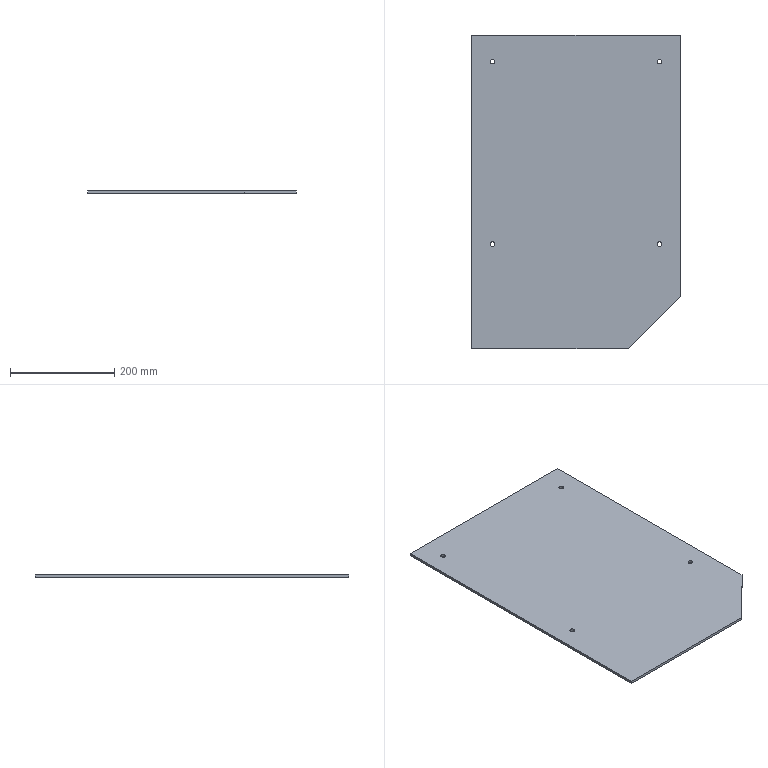Part | SolidWorks | features Chamfer 1, Extrusion 1, ICE 1 | 1 solid | 15 faces | box 400 x 600 x 5 mm | volume 1173728 mm3 | cylinder 8 | plane 7 | commonest cylinder face diameters 9 x8
STEP:
#1=CARTESIAN_POINT('',(-164.5,-100.,0.));
#2=VERTEX_POINT('',#1);
#3=CARTESIAN_POINT('',(-155.5,-100.,0.));
#4=VERTEX_POINT('',#3);
#5=CARTESIAN_POINT('',(-160.,-100.,0.));
#6=DIRECTION('',(0.,0.,1.));
#7=DIRECTION('',(1.,0.,0.));
#8=AXIS2_PLACEMENT_3D('',#5,#6,#7);
#9=CIRCLE('',#8,4.5);
#10=EDGE_CURVE('',#2,#4,#9,.T.);
#11=ORIENTED_EDGE('',*,*,#10,.F.);
#12=CARTESIAN_POINT('',(-164.5,-100.,5.));
#13=VERTEX_POINT('',#12);
#14=CARTESIAN_POINT('',(-164.5,-100.,0.));
#15=DIRECTION('',(0.,0.,1.));
#16=VECTOR('',#15,1000.);
#17=LINE('',#14,#16);
#18=EDGE_CURVE('',#2,#13,#17,.T.);
#19=ORIENTED_EDGE('',*,*,#18,.T.);
#20=CARTESIAN_POINT('',(-155.5,-100.,5.));
#21=VERTEX_POINT('',#20);
#22=CARTESIAN_POINT('',(-160.,-100.,5.));
#23=DIRECTION('',(0.,0.,1.));
#24=DIRECTION('',(1.,0.,0.));
#25=AXIS2_PLACEMENT_3D('',#22,#23,#24);
#26=CIRCLE('',#25,4.5);
#27=EDGE_CURVE('',#13,#21,#26,.T.);
#28=ORIENTED_EDGE('',*,*,#27,.T.);
#29=CARTESIAN_POINT('',(-155.5,-100.,0.));
#30=DIRECTION('',(0.,0.,1.));
#31=VECTOR('',#30,1000.);
#32=LINE('',#29,#31);
#33=EDGE_CURVE('',#4,#21,#32,.T.);
#34=ORIENTED_EDGE('',*,*,#33,.F.);
#35=EDGE_LOOP('',(#11,#19,#28,#34));
#36=FACE_OUTER_BOUND('',#35,.T.);
#37=CARTESIAN_POINT('',(-160.,-100.,0.));
#38=DIRECTION('',(0.,0.,1.));
#39=DIRECTION('',(1.,0.,0.));
#40=AXIS2_PLACEMENT_3D('',#37,#38,#39);
#41=CYLINDRICAL_SURFACE('',#40,4.5);
#42=ADVANCED_FACE('',(#36),#41,.F.);
#43=CARTESIAN_POINT('',(155.5,-100.,0.));
#44=VERTEX_POINT('',#43);
#45=CARTESIAN_POINT('',(164.5,-100.,0.));
#46=VERTEX_POINT('',#45);
#47=CARTESIAN_POINT('',(160.,-100.,0.));
#48=DIRECTION('',(0.,0.,1.));
#49=DIRECTION('',(1.,0.,0.));
#50=AXIS2_PLACEMENT_3D('',#47,#48,#49);
#51=CIRCLE('',#50,4.5);
#52=EDGE_CURVE('',#44,#46,#51,.T.);
#53=ORIENTED_EDGE('',*,*,#52,.F.);
#54=CARTESIAN_POINT('',(155.5,-100.,5.));
#55=VERTEX_POINT('',#54);
#56=CARTESIAN_POINT('',(155.5,-100.,0.));
#57=DIRECTION('',(0.,0.,1.));
#58=VECTOR('',#57,1000.);
#59=LINE('',#56,#58);
#60=EDGE_CURVE('',#44,#55,#59,.T.);
#61=ORIENTED_EDGE('',*,*,#60,.T.);
#62=CARTESIAN_POINT('',(164.5,-100.,5.));
#63=VERTEX_POINT('',#62);
#64=CARTESIAN_POINT('',(160.,-100.,5.));
#65=DIRECTION('',(0.,0.,1.));
#66=DIRECTION('',(1.,0.,0.));
#67=AXIS2_PLACEMENT_3D('',#64,#65,#66);
#68=CIRCLE('',#67,4.5);
#69=EDGE_CURVE('',#55,#63,#68,.T.);
#70=ORIENTED_EDGE('',*,*,#69,.T.);
#71=CARTESIAN_POINT('',(164.5,-100.,0.));
#72=DIRECTION('',(0.,0.,1.));
#73=VECTOR('',#72,1000.);
#74=LINE('',#71,#73);
#75=EDGE_CURVE('',#46,#63,#74,.T.);
#76=ORIENTED_EDGE('',*,*,#75,.F.);
#77=EDGE_LOOP('',(#53,#61,#70,#76));
#78=FACE_OUTER_BOUND('',#77,.T.);
#79=CARTESIAN_POINT('',(160.,-100.,0.));
#80=DIRECTION('',(0.,0.,1.));
#81=DIRECTION('',(1.,0.,0.));
#82=AXIS2_PLACEMENT_3D('',#79,#80,#81);
#83=CYLINDRICAL_SURFACE('',#82,4.5);
#84=ADVANCED_FACE('',(#78),#83,.F.);
#85=CARTESIAN_POINT('',(155.5,250.,0.));
#86=VERTEX_POINT('',#85);
#87=CARTESIAN_POINT('',(164.5,250.,0.));
#88=VERTEX_POINT('',#87);
#89=CARTESIAN_POINT('',(160.,250.,0.));
#90=DIRECTION('',(0.,0.,1.));
#91=DIRECTION('',(1.,0.,0.));
#92=AXIS2_PLACEMENT_3D('',#89,#90,#91);
#93=CIRCLE('',#92,4.5);
#94=EDGE_CURVE('',#86,#88,#93,.T.);
#95=ORIENTED_EDGE('',*,*,#94,.F.);
#96=CARTESIAN_POINT('',(155.5,250.,5.));
#97=VERTEX_POINT('',#96);
#98=CARTESIAN_POINT('',(155.5,250.,0.));
#99=DIRECTION('',(0.,0.,1.));
#100=VECTOR('',#99,1000.);
#101=LINE('',#98,#100);
#102=EDGE_CURVE('',#86,#97,#101,.T.);
#103=ORIENTED_EDGE('',*,*,#102,.T.);
#104=CARTESIAN_POINT('',(164.5,250.,5.));
#105=VERTEX_POINT('',#104);
#106=CARTESIAN_POINT('',(160.,250.,5.));
#107=DIRECTION('',(0.,0.,1.));
#108=DIRECTION('',(1.,0.,0.));
#109=AXIS2_PLACEMENT_3D('',#106,#107,#108);
#110=CIRCLE('',#109,4.5);
#111=EDGE_CURVE('',#97,#105,#110,.T.);
#112=ORIENTED_EDGE('',*,*,#111,.T.);
#113=CARTESIAN_POINT('',(164.5,250.,0.));
#114=DIRECTION('',(0.,0.,1.));
#115=VECTOR('',#114,1000.);
#116=LINE('',#113,#115);
#117=EDGE_CURVE('',#88,#105,#116,.T.);
#118=ORIENTED_EDGE('',*,*,#117,.F.);
#119=EDGE_LOOP('',(#95,#103,#112,#118));
#120=FACE_OUTER_BOUND('',#119,.T.);
#121=CARTESIAN_POINT('',(160.,250.,0.));
#122=DIRECTION('',(0.,0.,1.));
#123=DIRECTION('',(1.,0.,0.));
#124=AXIS2_PLACEMENT_3D('',#121,#122,#123);
#125=CYLINDRICAL_SURFACE('',#124,4.5);
#126=ADVANCED_FACE('',(#120),#125,.F.);
#127=CARTESIAN_POINT('',(-164.5,250.,0.));
#128=VERTEX_POINT('',#127);
#129=CARTESIAN_POINT('',(-155.5,250.,0.));
#130=VERTEX_POINT('',#129);
#131=CARTESIAN_POINT('',(-160.,250.,0.));
#132=DIRECTION('',(0.,0.,1.));
#133=DIRECTION('',(1.,0.,0.));
#134=AXIS2_PLACEMENT_3D('',#131,#132,#133);
#135=CIRCLE('',#134,4.5);
#136=EDGE_CURVE('',#128,#130,#135,.T.);
#137=ORIENTED_EDGE('',*,*,#136,.F.);
#138=CARTESIAN_POINT('',(-164.5,250.,5.));
#139=VERTEX_POINT('',#138);
#140=CARTESIAN_POINT('',(-164.5,250.,0.));
#141=DIRECTION('',(0.,0.,1.));
#142=VECTOR('',#141,1000.);
#143=LINE('',#140,#142);
#144=EDGE_CURVE('',#128,#139,#143,.T.);
#145=ORIENTED_EDGE('',*,*,#144,.T.);
#146=CARTESIAN_POINT('',(-155.5,250.,5.));
#147=VERTEX_POINT('',#146);
#148=CARTESIAN_POINT('',(-160.,250.,5.));
#149=DIRECTION('',(0.,0.,1.));
#150=DIRECTION('',(1.,0.,0.));
#151=AXIS2_PLACEMENT_3D('',#148,#149,#150);
#152=CIRCLE('',#151,4.5);
#153=EDGE_CURVE('',#139,#147,#152,.T.);
#154=ORIENTED_EDGE('',*,*,#153,.T.);
#155=CARTESIAN_POINT('',(-155.5,250.,0.));
#156=DIRECTION('',(0.,0.,1.));
#157=VECTOR('',#156,1000.);
#158=LINE('',#155,#157);
#159=EDGE_CURVE('',#130,#147,#158,.T.);
#160=ORIENTED_EDGE('',*,*,#159,.F.);
#161=EDGE_LOOP('',(#137,#145,#154,#160));
#162=FACE_OUTER_BOUND('',#161,.T.);
#163=CARTESIAN_POINT('',(-160.,250.,0.));
#164=DIRECTION('',(0.,0.,1.));
#165=DIRECTION('',(1.,0.,0.));
#166=AXIS2_PLACEMENT_3D('',#163,#164,#165);
#167=CYLINDRICAL_SURFACE('',#166,4.5);
#168=ADVANCED_FACE('',(#162),#167,.F.);
#169=CARTESIAN_POINT('',(200.,-200.,5.));
#170=VERTEX_POINT('',#169);
#171=CARTESIAN_POINT('',(200.,300.,5.));
#172=VERTEX_POINT('',#171);
#173=CARTESIAN_POINT('',(200.,-300.,5.));
#174=DIRECTION('',(0.,1.,0.));
#175=VECTOR('',#174,1000.);
#176=LINE('',#173,#175);
#177=EDGE_CURVE('',#170,#172,#176,.T.);
#178=ORIENTED_EDGE('',*,*,#177,.F.);
#179=CARTESIAN_POINT('',(200.,-200.,0.));
#180=VERTEX_POINT('',#179);
#181=CARTESIAN_POINT('',(200.,-200.,5.));
#182=DIRECTION('',(0.,0.,-1.));
#183=VECTOR('',#182,1000.);
#184=LINE('',#181,#183);
#185=EDGE_CURVE('',#170,#180,#184,.T.);
#186=ORIENTED_EDGE('',*,*,#185,.T.);
#187=CARTESIAN_POINT('',(200.,300.,0.));
#188=VERTEX_POINT('',#187);
#189=CARTESIAN_POINT('',(200.,-300.,0.));
#190=DIRECTION('',(0.,1.,0.));
#191=VECTOR('',#190,1000.);
#192=LINE('',#189,#191);
#193=EDGE_CURVE('',#180,#188,#192,.T.);
#194=ORIENTED_EDGE('',*,*,#193,.T.);
#195=CARTESIAN_POINT('',(200.,300.,5.));
#196=DIRECTION('',(0.,0.,-1.));
#197=VECTOR('',#196,1000.);
#198=LINE('',#195,#197);
#199=EDGE_CURVE('',#172,#188,#198,.T.);
#200=ORIENTED_EDGE('',*,*,#199,.F.);
#201=EDGE_LOOP('',(#178,#186,#194,#200));
#202=FACE_OUTER_BOUND('',#201,.T.);
#203=CARTESIAN_POINT('',(200.,-300.,5.));
#204=DIRECTION('',(-1.,0.,0.));
#205=DIRECTION('',(0.,0.,1.));
#206=AXIS2_PLACEMENT_3D('',#203,#204,#205);
#207=PLANE('',#206);
#208=ADVANCED_FACE('',(#202),#207,.F.);
#209=CARTESIAN_POINT('',(-200.,300.,0.));
#210=VERTEX_POINT('',#209);
#211=CARTESIAN_POINT('',(-200.,300.,0.));
#212=DIRECTION('',(-1.,0.,0.));
#213=VECTOR('',#212,1000.);
#214=LINE('',#211,#213);
#215=EDGE_CURVE('',#188,#210,#214,.T.);
#216=ORIENTED_EDGE('',*,*,#215,.T.);
#217=CARTESIAN_POINT('',(-200.,300.,5.));
#218=VERTEX_POINT('',#217);
#219=CARTESIAN_POINT('',(-200.,300.,5.));
#220=DIRECTION('',(0.,0.,-1.));
#221=VECTOR('',#220,1000.);
#222=LINE('',#219,#221);
#223=EDGE_CURVE('',#218,#210,#222,.T.);
#224=ORIENTED_EDGE('',*,*,#223,.F.);
#225=CARTESIAN_POINT('',(-200.,300.,5.));
#226=DIRECTION('',(-1.,0.,0.));
#227=VECTOR('',#226,1000.);
#228=LINE('',#225,#227);
#229=EDGE_CURVE('',#172,#218,#228,.T.);
#230=ORIENTED_EDGE('',*,*,#229,.F.);
#231=ORIENTED_EDGE('',*,*,#199,.T.);
#232=EDGE_LOOP('',(#216,#224,#230,#231));
#233=FACE_OUTER_BOUND('',#232,.T.);
#234=CARTESIAN_POINT('',(-200.,300.,5.));
#235=DIRECTION('',(0.,-1.,0.));
#236=DIRECTION('',(0.,0.,-1.));
#237=AXIS2_PLACEMENT_3D('',#234,#235,#236);
#238=PLANE('',#237);
#239=ADVANCED_FACE('',(#233),#238,.F.);
#240=CARTESIAN_POINT('',(-200.,-300.,0.));
#241=VERTEX_POINT('',#240);
#242=CARTESIAN_POINT('',(-200.,-300.,0.));
#243=DIRECTION('',(0.,-1.,0.));
#244=VECTOR('',#243,1000.);
#245=LINE('',#242,#244);
#246=EDGE_CURVE('',#210,#241,#245,.T.);
#247=ORIENTED_EDGE('',*,*,#246,.T.);
#248=CARTESIAN_POINT('',(-200.,-300.,5.));
#249=VERTEX_POINT('',#248);
#250=CARTESIAN_POINT('',(-200.,-300.,5.));
#251=DIRECTION('',(0.,0.,-1.));
#252=VECTOR('',#251,1000.);
#253=LINE('',#250,#252);
#254=EDGE_CURVE('',#249,#241,#253,.T.);
#255=ORIENTED_EDGE('',*,*,#254,.F.);
#256=CARTESIAN_POINT('',(-200.,-300.,5.));
#257=DIRECTION('',(0.,-1.,0.));
#258=VECTOR('',#257,1000.);
#259=LINE('',#256,#258);
#260=EDGE_CURVE('',#218,#249,#259,.T.);
#261=ORIENTED_EDGE('',*,*,#260,.F.);
#262=ORIENTED_EDGE('',*,*,#223,.T.);
#263=EDGE_LOOP('',(#247,#255,#261,#262));
#264=FACE_OUTER_BOUND('',#263,.T.);
#265=CARTESIAN_POINT('',(-200.,-300.,5.));
#266=DIRECTION('',(1.,0.,0.));
#267=DIRECTION('',(0.,0.,-1.));
#268=AXIS2_PLACEMENT_3D('',#265,#266,#267);
#269=PLANE('',#268);
#270=ADVANCED_FACE('',(#264),#269,.F.);
#271=CARTESIAN_POINT('',(100.,-300.,0.));
#272=VERTEX_POINT('',#271);
#273=CARTESIAN_POINT('',(-200.,-300.,0.));
#274=DIRECTION('',(1.,0.,0.));
#275=VECTOR('',#274,1000.);
#276=LINE('',#273,#275);
#277=EDGE_CURVE('',#241,#272,#276,.T.);
#278=ORIENTED_EDGE('',*,*,#277,.T.);
#279=CARTESIAN_POINT('',(100.,-300.,5.));
#280=VERTEX_POINT('',#279);
#281=CARTESIAN_POINT('',(100.,-300.,5.));
#282=DIRECTION('',(0.,0.,1.));
#283=VECTOR('',#282,1000.);
#284=LINE('',#281,#283);
#285=EDGE_CURVE('',#272,#280,#284,.T.);
#286=ORIENTED_EDGE('',*,*,#285,.T.);
#287=CARTESIAN_POINT('',(-200.,-300.,5.));
#288=DIRECTION('',(1.,0.,0.));
#289=VECTOR('',#288,1000.);
#290=LINE('',#287,#289);
#291=EDGE_CURVE('',#249,#280,#290,.T.);
#292=ORIENTED_EDGE('',*,*,#291,.F.);
#293=ORIENTED_EDGE('',*,*,#254,.T.);
#294=EDGE_LOOP('',(#278,#286,#292,#293));
#295=FACE_OUTER_BOUND('',#294,.T.);
#296=CARTESIAN_POINT('',(-200.,-300.,5.));
#297=DIRECTION('',(0.,1.,0.));
#298=DIRECTION('',(0.,0.,1.));
#299=AXIS2_PLACEMENT_3D('',#296,#297,#298);
#300=PLANE('',#299);
#301=ADVANCED_FACE('',(#295),#300,.F.);
#302=CARTESIAN_POINT('',(-160.,-100.,5.));
#303=DIRECTION('',(0.,0.,1.));
#304=DIRECTION('',(1.,0.,0.));
#305=AXIS2_PLACEMENT_3D('',#302,#303,#304);
#306=CIRCLE('',#305,4.5);
#307=EDGE_CURVE('',#21,#13,#306,.T.);
#308=ORIENTED_EDGE('',*,*,#307,.F.);
#309=ORIENTED_EDGE('',*,*,#27,.F.);
#310=EDGE_LOOP('',(#308,#309));
#311=FACE_BOUND('',#310,.T.);
#312=CARTESIAN_POINT('',(160.,-100.,5.));
#313=DIRECTION('',(0.,0.,1.));
#314=DIRECTION('',(1.,0.,0.));
#315=AXIS2_PLACEMENT_3D('',#312,#313,#314);
#316=CIRCLE('',#315,4.5);
#317=EDGE_CURVE('',#63,#55,#316,.T.);
#318=ORIENTED_EDGE('',*,*,#317,.F.);
#319=ORIENTED_EDGE('',*,*,#69,.F.);
#320=EDGE_LOOP('',(#318,#319));
#321=FACE_BOUND('',#320,.T.);
#322=CARTESIAN_POINT('',(160.,250.,5.));
#323=DIRECTION('',(0.,0.,1.));
#324=DIRECTION('',(1.,0.,0.));
#325=AXIS2_PLACEMENT_3D('',#322,#323,#324);
#326=CIRCLE('',#325,4.5);
#327=EDGE_CURVE('',#105,#97,#326,.T.);
#328=ORIENTED_EDGE('',*,*,#327,.F.);
#329=ORIENTED_EDGE('',*,*,#111,.F.);
#330=EDGE_LOOP('',(#328,#329));
#331=FACE_BOUND('',#330,.T.);
#332=CARTESIAN_POINT('',(-160.,250.,5.));
#333=DIRECTION('',(0.,0.,1.));
#334=DIRECTION('',(1.,0.,0.));
#335=AXIS2_PLACEMENT_3D('',#332,#333,#334);
#336=CIRCLE('',#335,4.5);
#337=EDGE_CURVE('',#147,#139,#336,.T.);
#338=ORIENTED_EDGE('',*,*,#337,.F.);
#339=ORIENTED_EDGE('',*,*,#153,.F.);
#340=EDGE_LOOP('',(#338,#339));
#341=FACE_BOUND('',#340,.T.);
#342=ORIENTED_EDGE('',*,*,#291,.T.);
#343=CARTESIAN_POINT('',(200.,-200.,5.));
#344=DIRECTION('',(0.7071,0.7071,0.));
#345=VECTOR('',#344,1000.);
#346=LINE('',#343,#345);
#347=EDGE_CURVE('',#280,#170,#346,.T.);
#348=ORIENTED_EDGE('',*,*,#347,.T.);
#349=ORIENTED_EDGE('',*,*,#177,.T.);
#350=ORIENTED_EDGE('',*,*,#229,.T.);
#351=ORIENTED_EDGE('',*,*,#260,.T.);
#352=EDGE_LOOP('',(#342,#348,#349,#350,#351));
#353=FACE_OUTER_BOUND('',#352,.T.);
#354=CARTESIAN_POINT('',(0.,0.,5.));
#355=DIRECTION('',(0.,0.,-1.));
#356=DIRECTION('',(-1.,0.,0.));
#357=AXIS2_PLACEMENT_3D('',#354,#355,#356);
#358=PLANE('',#357);
#359=ADVANCED_FACE('',(#311,#321,#331,#341,#353),#358,.F.);
#360=CARTESIAN_POINT('',(-160.,-100.,0.));
#361=DIRECTION('',(0.,0.,1.));
#362=DIRECTION('',(1.,0.,0.));
#363=AXIS2_PLACEMENT_3D('',#360,#361,#362);
#364=CIRCLE('',#363,4.5);
#365=EDGE_CURVE('',#4,#2,#364,.T.);
#366=ORIENTED_EDGE('',*,*,#365,.T.);
#367=ORIENTED_EDGE('',*,*,#10,.T.);
#368=EDGE_LOOP('',(#366,#367));
#369=FACE_BOUND('',#368,.T.);
#370=CARTESIAN_POINT('',(160.,-100.,0.));
#371=DIRECTION('',(0.,0.,1.));
#372=DIRECTION('',(1.,0.,0.));
#373=AXIS2_PLACEMENT_3D('',#370,#371,#372);
#374=CIRCLE('',#373,4.5);
#375=EDGE_CURVE('',#46,#44,#374,.T.);
#376=ORIENTED_EDGE('',*,*,#375,.T.);
#377=ORIENTED_EDGE('',*,*,#52,.T.);
#378=EDGE_LOOP('',(#376,#377));
#379=FACE_BOUND('',#378,.T.);
#380=CARTESIAN_POINT('',(160.,250.,0.));
#381=DIRECTION('',(0.,0.,1.));
#382=DIRECTION('',(1.,0.,0.));
#383=AXIS2_PLACEMENT_3D('',#380,#381,#382);
#384=CIRCLE('',#383,4.5);
#385=EDGE_CURVE('',#88,#86,#384,.T.);
#386=ORIENTED_EDGE('',*,*,#385,.T.);
#387=ORIENTED_EDGE('',*,*,#94,.T.);
#388=EDGE_LOOP('',(#386,#387));
#389=FACE_BOUND('',#388,.T.);
#390=CARTESIAN_POINT('',(-160.,250.,0.));
#391=DIRECTION('',(0.,0.,1.));
#392=DIRECTION('',(1.,0.,0.));
#393=AXIS2_PLACEMENT_3D('',#390,#391,#392);
#394=CIRCLE('',#393,4.5);
#395=EDGE_CURVE('',#130,#128,#394,.T.);
#396=ORIENTED_EDGE('',*,*,#395,.T.);
#397=ORIENTED_EDGE('',*,*,#136,.T.);
#398=EDGE_LOOP('',(#396,#397));
#399=FACE_BOUND('',#398,.T.);
#400=ORIENTED_EDGE('',*,*,#193,.F.);
#401=CARTESIAN_POINT('',(200.,-200.,0.));
#402=DIRECTION('',(-0.7071,-0.7071,0.));
#403=VECTOR('',#402,1000.);
#404=LINE('',#401,#403);
#405=EDGE_CURVE('',#180,#272,#404,.T.);
#406=ORIENTED_EDGE('',*,*,#405,.T.);
#407=ORIENTED_EDGE('',*,*,#277,.F.);
#408=ORIENTED_EDGE('',*,*,#246,.F.);
#409=ORIENTED_EDGE('',*,*,#215,.F.);
#410=EDGE_LOOP('',(#400,#406,#407,#408,#409));
#411=FACE_OUTER_BOUND('',#410,.T.);
#412=CARTESIAN_POINT('',(0.,0.,0.));
#413=DIRECTION('',(0.,0.,-1.));
#414=DIRECTION('',(-1.,0.,0.));
#415=AXIS2_PLACEMENT_3D('',#412,#413,#414);
#416=PLANE('',#415);
#417=ADVANCED_FACE('',(#369,#379,#389,#399,#411),#416,.T.);
#418=ORIENTED_EDGE('',*,*,#144,.F.);
#419=ORIENTED_EDGE('',*,*,#395,.F.);
#420=ORIENTED_EDGE('',*,*,#159,.T.);
#421=ORIENTED_EDGE('',*,*,#337,.T.);
#422=EDGE_LOOP('',(#418,#419,#420,#421));
#423=FACE_OUTER_BOUND('',#422,.T.);
#424=CARTESIAN_POINT('',(-160.,250.,0.));
#425=DIRECTION('',(0.,0.,1.));
#426=DIRECTION('',(1.,0.,0.));
#427=AXIS2_PLACEMENT_3D('',#424,#425,#426);
#428=CYLINDRICAL_SURFACE('',#427,4.5);
#429=ADVANCED_FACE('',(#423),#428,.F.);
#430=ORIENTED_EDGE('',*,*,#102,.F.);
#431=ORIENTED_EDGE('',*,*,#385,.F.);
#432=ORIENTED_EDGE('',*,*,#117,.T.);
#433=ORIENTED_EDGE('',*,*,#327,.T.);
#434=EDGE_LOOP('',(#430,#431,#432,#433));
#435=FACE_OUTER_BOUND('',#434,.T.);
#436=CARTESIAN_POINT('',(160.,250.,0.));
#437=DIRECTION('',(0.,0.,1.));
#438=DIRECTION('',(1.,0.,0.));
#439=AXIS2_PLACEMENT_3D('',#436,#437,#438);
#440=CYLINDRICAL_SURFACE('',#439,4.5);
#441=ADVANCED_FACE('',(#435),#440,.F.);
#442=ORIENTED_EDGE('',*,*,#60,.F.);
#443=ORIENTED_EDGE('',*,*,#375,.F.);
#444=ORIENTED_EDGE('',*,*,#75,.T.);
#445=ORIENTED_EDGE('',*,*,#317,.T.);
#446=EDGE_LOOP('',(#442,#443,#444,#445));
#447=FACE_OUTER_BOUND('',#446,.T.);
#448=CARTESIAN_POINT('',(160.,-100.,0.));
#449=DIRECTION('',(0.,0.,1.));
#450=DIRECTION('',(1.,0.,0.));
#451=AXIS2_PLACEMENT_3D('',#448,#449,#450);
#452=CYLINDRICAL_SURFACE('',#451,4.5);
#453=ADVANCED_FACE('',(#447),#452,.F.);
#454=ORIENTED_EDGE('',*,*,#18,.F.);
#455=ORIENTED_EDGE('',*,*,#365,.F.);
#456=ORIENTED_EDGE('',*,*,#33,.T.);
#457=ORIENTED_EDGE('',*,*,#307,.T.);
#458=EDGE_LOOP('',(#454,#455,#456,#457));
#459=FACE_OUTER_BOUND('',#458,.T.);
#460=CARTESIAN_POINT('',(-160.,-100.,0.));
#461=DIRECTION('',(0.,0.,1.));
#462=DIRECTION('',(1.,0.,0.));
#463=AXIS2_PLACEMENT_3D('',#460,#461,#462);
#464=CYLINDRICAL_SURFACE('',#463,4.5);
#465=ADVANCED_FACE('',(#459),#464,.F.);
#466=ORIENTED_EDGE('',*,*,#347,.F.);
#467=ORIENTED_EDGE('',*,*,#285,.F.);
#468=ORIENTED_EDGE('',*,*,#405,.F.);
#469=ORIENTED_EDGE('',*,*,#185,.F.);
#470=EDGE_LOOP('',(#466,#467,#468,#469));
#471=FACE_OUTER_BOUND('',#470,.T.);
#472=CARTESIAN_POINT('',(200.,-200.,5.));
#473=DIRECTION('',(-0.7071,0.7071,0.));
#474=DIRECTION('',(0.,0.,-1.));
#475=AXIS2_PLACEMENT_3D('',#472,#473,#474);
#476=PLANE('',#475);
#477=ADVANCED_FACE('',(#471),#476,.F.);
#478=CLOSED_SHELL('',(#42,#84,#126,#168,#208,#239,#270,#301,#359,#417,#429,#441,#453,#465,#477));
#479=MANIFOLD_SOLID_BREP('',#478);
#480=CARTESIAN_POINT('',(0.,0.,0.));
#481=DIRECTION('',(0.,0.,1.));
#482=DIRECTION('',(1.,0.,0.));
#483=AXIS2_PLACEMENT_3D('',#480,#481,#482);
#484=(LENGTH_UNIT()NAMED_UNIT(*)SI_UNIT(.MILLI.,.METRE.));
#485=UNCERTAINTY_MEASURE_WITH_UNIT(LENGTH_MEASURE(0.00001),#484,'','');
#486=(NAMED_UNIT(*)PLANE_ANGLE_UNIT()SI_UNIT($,.RADIAN.));
#487=(NAMED_UNIT(*)SI_UNIT($,.STERADIAN.)SOLID_ANGLE_UNIT());
#488=(GEOMETRIC_REPRESENTATION_CONTEXT(3)GLOBAL_UNCERTAINTY_ASSIGNED_CONTEXT((#485))GLOBAL_UNIT_ASSIGNED_CONTEXT((#484,#486,#487))REPRESENTATION_CONTEXT('',''));
#489=ADVANCED_BREP_SHAPE_REPRESENTATION('',(#479,#483),#488);